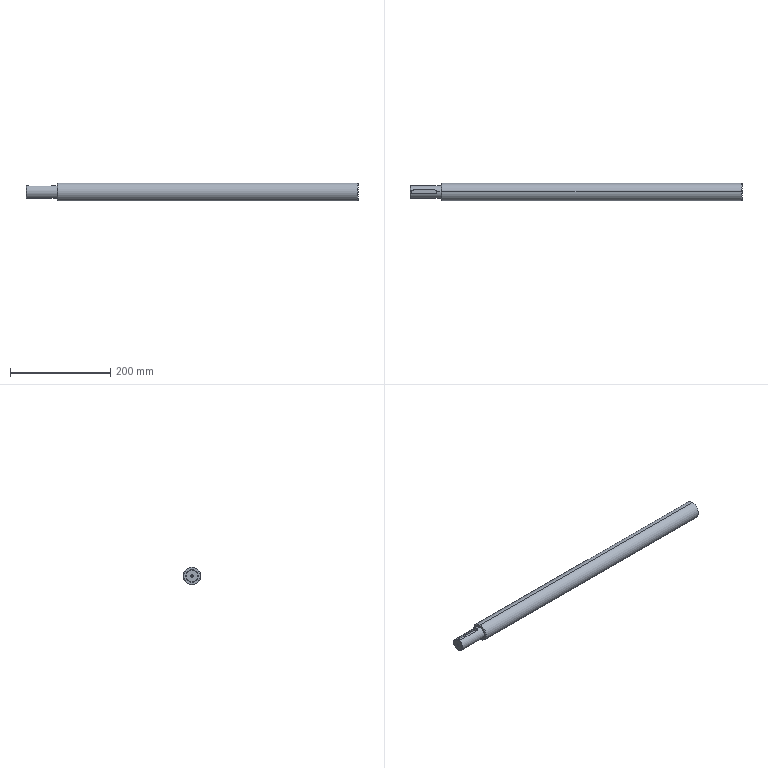Part | STEP file | PN_0055_driver shaft_default_machined_ | 1 solid | 23 faces | box 662 x 35 x 35 mm | volume 605787 mm3 | cylinder 9 | cone 8 | plane 6 | commonest cylinder face diameters 8 x3 5 x2 25 x2 35 x2